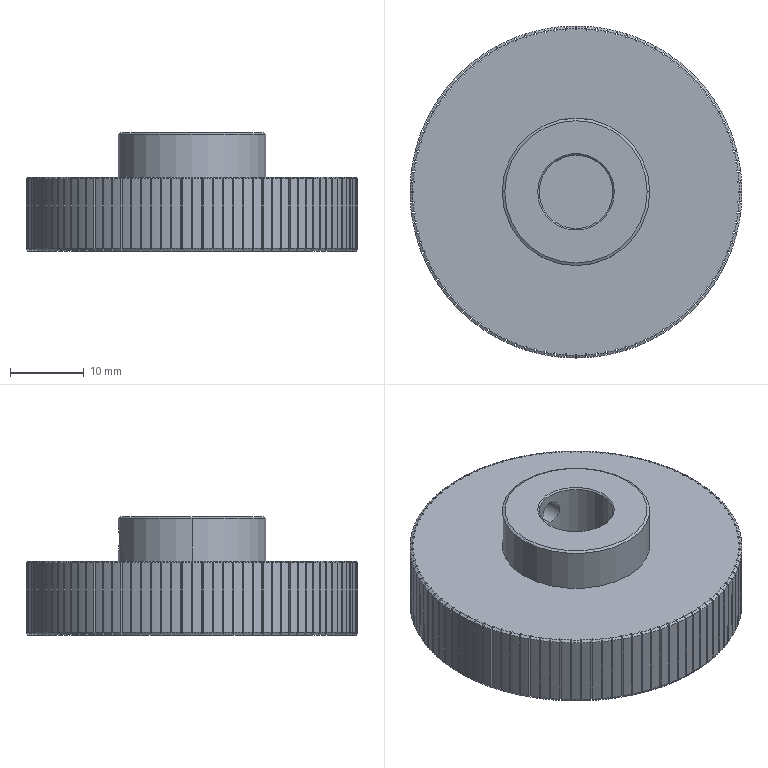Part | STEP file | FBDS-CS-021 | 1 solid | 617 faces | box 45 x 45 x 16 mm | volume 16300 mm3 | plane 305 | cone 204 | cylinder 108 | commonest cylinder face diameters 45 x100 3.3 x2 10 x2 20 x2 30 x2